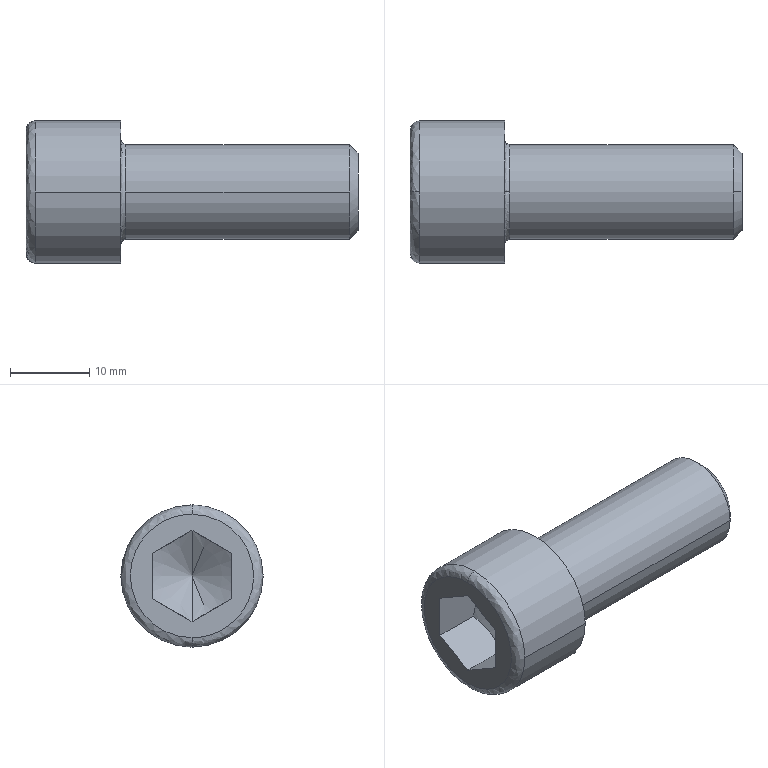Part | STEP file | Broached Socket Head Cap Screw - Metric M12x1.75 x 30 | 1 solid | 21 faces | box 42 x 18 x 18 mm | volume 5780 mm3 | plane 9 | spline 4 | cylinder 4 | cone 4 | commonest cylinder face diameters 12 x2 18 x2